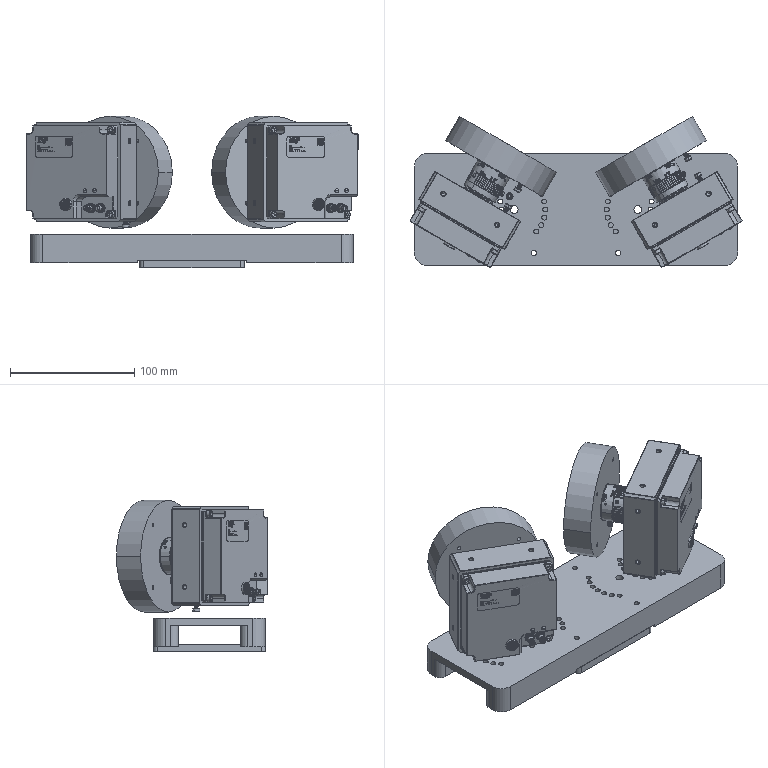Part | SolidWorks | 15 solids | 4145 faces | volume 1121716 mm3 | cylinder 1689 | plane 1546 | cone 542 | spline 256 | torus 92 | sphere 20 | commonest cylinder face diameters 1.113 x210 29.5 x200 4 x192 3 x170 2.5 x145 29.44 x50